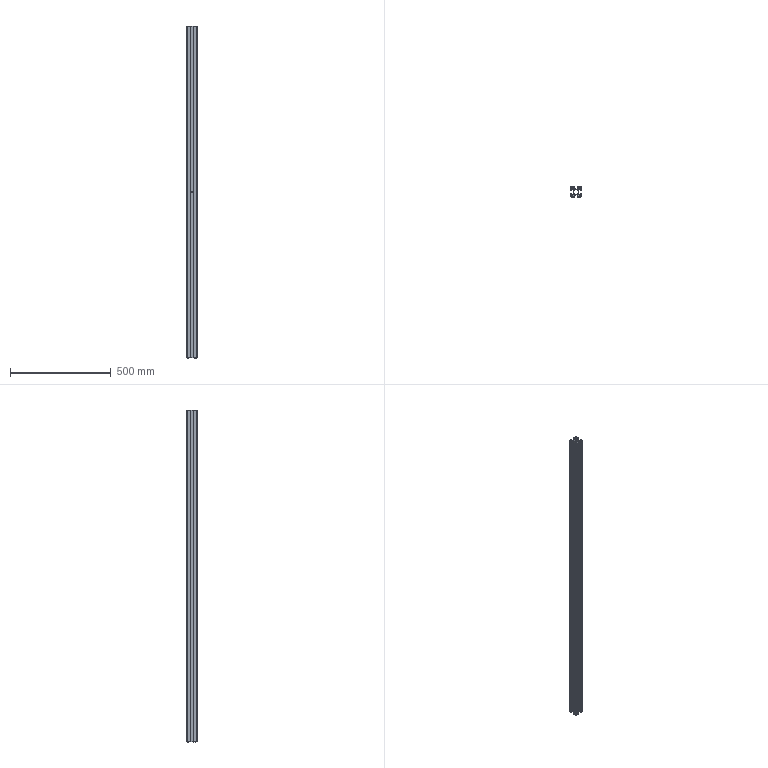Part | STEP file | 46A-00006CC11-1650mm | 1 solid | 146 faces | box 50 x 50 x 1650 mm | volume 969108 mm3 | cylinder 88 | plane 58 | commonest cylinder face diameters 1 x24 4 x24 1.5 x16 3.7 x8 6.7 x8 2 x4